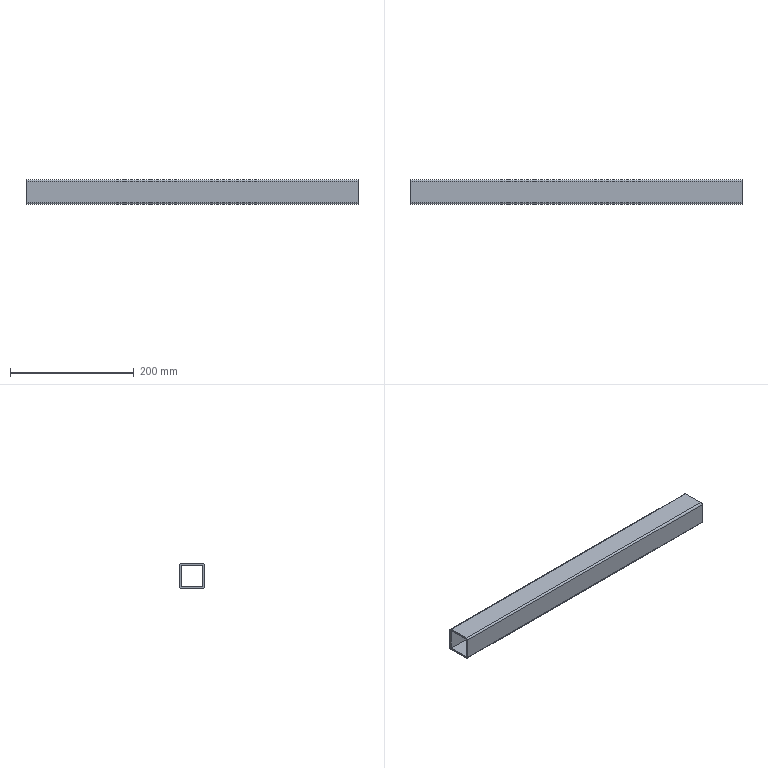Part | NX | features solid 2 | 1 solid | 28 faces | box 536 x 40 x 40 mm | volume 219712 mm3 | plane 24 | cylinder 4 | commonest cylinder face diameters 5.6 x4
STEP:
#1=CARTESIAN_POINT('',(-268.,-42.2,-355.7));
#2=VERTEX_POINT('',#1);
#3=CARTESIAN_POINT('',(-268.,-7.8,-355.7));
#4=VERTEX_POINT('',#3);
#5=CARTESIAN_POINT('',(-268.,-42.2,-355.7));
#6=DIRECTION('',(0.,1.,0.));
#7=VECTOR('',#6,1000.);
#8=LINE('',#5,#7);
#9=EDGE_CURVE('',#2,#4,#8,.T.);
#10=ORIENTED_EDGE('',*,*,#9,.T.);
#11=CARTESIAN_POINT('',(268.,-7.8,-355.7));
#12=VERTEX_POINT('',#11);
#13=CARTESIAN_POINT('',(-268.,-7.8,-355.7));
#14=DIRECTION('',(1.,0.,0.));
#15=VECTOR('',#14,1000.);
#16=LINE('',#13,#15);
#17=EDGE_CURVE('',#4,#12,#16,.T.);
#18=ORIENTED_EDGE('',*,*,#17,.T.);
#19=CARTESIAN_POINT('',(268.,-42.2,-355.7));
#20=VERTEX_POINT('',#19);
#21=CARTESIAN_POINT('',(268.,-42.2,-355.7));
#22=DIRECTION('',(0.,1.,0.));
#23=VECTOR('',#22,1000.);
#24=LINE('',#21,#23);
#25=EDGE_CURVE('',#20,#12,#24,.T.);
#26=ORIENTED_EDGE('',*,*,#25,.F.);
#27=CARTESIAN_POINT('',(268.,-42.2,-355.7));
#28=DIRECTION('',(-1.,0.,0.));
#29=VECTOR('',#28,1000.);
#30=LINE('',#27,#29);
#31=EDGE_CURVE('',#20,#2,#30,.T.);
#32=ORIENTED_EDGE('',*,*,#31,.T.);
#33=EDGE_LOOP('',(#10,#18,#26,#32));
#34=FACE_BOUND('',#33,.T.);
#35=CARTESIAN_POINT('',(-268.,-45.,-355.7));
#36=DIRECTION('',(0.,0.,-1.));
#37=DIRECTION('',(0.,-1.,0.));
#38=AXIS2_PLACEMENT_3D('',#35,#36,#37);
#39=PLANE('',#38);
#40=ADVANCED_FACE('',(#34),#39,.T.);
#41=CARTESIAN_POINT('',(-268.,-45.,-352.9));
#42=VERTEX_POINT('',#41);
#43=CARTESIAN_POINT('',(-268.,-42.2,-352.9));
#44=DIRECTION('',(1.,0.,0.));
#45=DIRECTION('',(0.,-1.,0.));
#46=AXIS2_PLACEMENT_3D('',#43,#44,#45);
#47=CIRCLE('',#46,2.8);
#48=EDGE_CURVE('',#42,#2,#47,.T.);
#49=ORIENTED_EDGE('',*,*,#48,.T.);
#50=ORIENTED_EDGE('',*,*,#31,.F.);
#51=CARTESIAN_POINT('',(268.,-45.,-352.9));
#52=VERTEX_POINT('',#51);
#53=CARTESIAN_POINT('',(268.,-42.2,-352.9));
#54=DIRECTION('',(-1.,0.,0.));
#55=DIRECTION('',(0.,0.,-1.));
#56=AXIS2_PLACEMENT_3D('',#53,#54,#55);
#57=CIRCLE('',#56,2.8);
#58=EDGE_CURVE('',#20,#52,#57,.T.);
#59=ORIENTED_EDGE('',*,*,#58,.T.);
#60=CARTESIAN_POINT('',(-268.,-45.,-352.9));
#61=DIRECTION('',(1.,0.,0.));
#62=VECTOR('',#61,1000.);
#63=LINE('',#60,#62);
#64=EDGE_CURVE('',#42,#52,#63,.T.);
#65=ORIENTED_EDGE('',*,*,#64,.F.);
#66=EDGE_LOOP('',(#49,#50,#59,#65));
#67=FACE_BOUND('',#66,.T.);
#68=CARTESIAN_POINT('',(966.73,-42.2,-352.9));
#69=DIRECTION('',(-1.,0.,0.));
#70=DIRECTION('',(0.,0.,1.));
#71=AXIS2_PLACEMENT_3D('',#68,#69,#70);
#72=CYLINDRICAL_SURFACE('',#71,2.8);
#73=ADVANCED_FACE('',(#67),#72,.T.);
#74=CARTESIAN_POINT('',(268.,-45.,-318.5));
#75=VERTEX_POINT('',#74);
#76=CARTESIAN_POINT('',(268.,-45.,-318.5));
#77=DIRECTION('',(0.,0.,-1.));
#78=VECTOR('',#77,1000.);
#79=LINE('',#76,#78);
#80=EDGE_CURVE('',#75,#52,#79,.T.);
#81=ORIENTED_EDGE('',*,*,#80,.F.);
#82=CARTESIAN_POINT('',(-268.,-45.,-318.5));
#83=VERTEX_POINT('',#82);
#84=CARTESIAN_POINT('',(268.,-45.,-318.5));
#85=DIRECTION('',(-1.,0.,0.));
#86=VECTOR('',#85,1000.);
#87=LINE('',#84,#86);
#88=EDGE_CURVE('',#75,#83,#87,.T.);
#89=ORIENTED_EDGE('',*,*,#88,.T.);
#90=CARTESIAN_POINT('',(-268.,-45.,-318.5));
#91=DIRECTION('',(0.,0.,-1.));
#92=VECTOR('',#91,1000.);
#93=LINE('',#90,#92);
#94=EDGE_CURVE('',#83,#42,#93,.T.);
#95=ORIENTED_EDGE('',*,*,#94,.T.);
#96=ORIENTED_EDGE('',*,*,#64,.T.);
#97=EDGE_LOOP('',(#81,#89,#95,#96));
#98=FACE_BOUND('',#97,.T.);
#99=CARTESIAN_POINT('',(-268.,-45.,-315.7));
#100=DIRECTION('',(0.,-1.,0.));
#101=DIRECTION('',(0.,0.,1.));
#102=AXIS2_PLACEMENT_3D('',#99,#100,#101);
#103=PLANE('',#102);
#104=ADVANCED_FACE('',(#98),#103,.T.);
#105=ORIENTED_EDGE('',*,*,#94,.F.);
#106=CARTESIAN_POINT('',(-268.,-42.2,-318.5));
#107=VERTEX_POINT('',#106);
#108=CARTESIAN_POINT('',(-268.,-45.,-318.5));
#109=DIRECTION('',(0.,1.,0.));
#110=VECTOR('',#109,1000.);
#111=LINE('',#108,#110);
#112=EDGE_CURVE('',#83,#107,#111,.T.);
#113=ORIENTED_EDGE('',*,*,#112,.T.);
#114=CARTESIAN_POINT('',(-268.,-42.2,-352.9));
#115=VERTEX_POINT('',#114);
#116=CARTESIAN_POINT('',(-268.,-42.2,-318.5));
#117=DIRECTION('',(0.,0.,-1.));
#118=VECTOR('',#117,1000.);
#119=LINE('',#116,#118);
#120=EDGE_CURVE('',#107,#115,#119,.T.);
#121=ORIENTED_EDGE('',*,*,#120,.T.);
#122=CARTESIAN_POINT('',(-268.,-45.,-352.9));
#123=DIRECTION('',(0.,1.,0.));
#124=VECTOR('',#123,1000.);
#125=LINE('',#122,#124);
#126=EDGE_CURVE('',#42,#115,#125,.T.);
#127=ORIENTED_EDGE('',*,*,#126,.F.);
#128=EDGE_LOOP('',(#105,#113,#121,#127));
#129=FACE_BOUND('',#128,.T.);
#130=CARTESIAN_POINT('',(-268.,-43.6,-335.7));
#131=DIRECTION('',(-1.,0.,0.));
#132=DIRECTION('',(0.,0.,1.));
#133=AXIS2_PLACEMENT_3D('',#130,#131,#132);
#134=PLANE('',#133);
#135=ADVANCED_FACE('',(#129),#134,.T.);
#136=ORIENTED_EDGE('',*,*,#126,.T.);
#137=CARTESIAN_POINT('',(-268.,-42.2,-355.7));
#138=DIRECTION('',(0.,0.,1.));
#139=VECTOR('',#138,1000.);
#140=LINE('',#137,#139);
#141=EDGE_CURVE('',#2,#115,#140,.T.);
#142=ORIENTED_EDGE('',*,*,#141,.F.);
#143=ORIENTED_EDGE('',*,*,#48,.F.);
#144=EDGE_LOOP('',(#136,#142,#143));
#145=FACE_BOUND('',#144,.T.);
#146=CARTESIAN_POINT('',(-268.,-43.19,-353.89));
#147=DIRECTION('',(1.,0.,0.));
#148=DIRECTION('',(0.,1.,0.));
#149=AXIS2_PLACEMENT_3D('',#146,#147,#148);
#150=PLANE('',#149);
#151=ADVANCED_FACE('',(#145),#150,.F.);
#152=ORIENTED_EDGE('',*,*,#9,.F.);
#153=ORIENTED_EDGE('',*,*,#141,.T.);
#154=CARTESIAN_POINT('',(-268.,-7.8,-352.9));
#155=VERTEX_POINT('',#154);
#156=CARTESIAN_POINT('',(-268.,-42.2,-352.9));
#157=DIRECTION('',(0.,1.,0.));
#158=VECTOR('',#157,1000.);
#159=LINE('',#156,#158);
#160=EDGE_CURVE('',#115,#155,#159,.T.);
#161=ORIENTED_EDGE('',*,*,#160,.T.);
#162=CARTESIAN_POINT('',(-268.,-7.8,-355.7));
#163=DIRECTION('',(0.,0.,1.));
#164=VECTOR('',#163,1000.);
#165=LINE('',#162,#164);
#166=EDGE_CURVE('',#4,#155,#165,.T.);
#167=ORIENTED_EDGE('',*,*,#166,.F.);
#168=EDGE_LOOP('',(#152,#153,#161,#167));
#169=FACE_BOUND('',#168,.T.);
#170=CARTESIAN_POINT('',(-268.,-25.,-354.3));
#171=DIRECTION('',(-1.,0.,0.));
#172=DIRECTION('',(0.,-1.,0.));
#173=AXIS2_PLACEMENT_3D('',#170,#171,#172);
#174=PLANE('',#173);
#175=ADVANCED_FACE('',(#169),#174,.T.);
#176=ORIENTED_EDGE('',*,*,#166,.T.);
#177=CARTESIAN_POINT('',(-268.,-5.,-352.9));
#178=VERTEX_POINT('',#177);
#179=CARTESIAN_POINT('',(-268.,-5.,-352.9));
#180=DIRECTION('',(0.,-1.,0.));
#181=VECTOR('',#180,1000.);
#182=LINE('',#179,#181);
#183=EDGE_CURVE('',#178,#155,#182,.T.);
#184=ORIENTED_EDGE('',*,*,#183,.F.);
#185=CARTESIAN_POINT('',(-268.,-7.8,-352.9));
#186=DIRECTION('',(1.,0.,0.));
#187=DIRECTION('',(0.,0.,-1.));
#188=AXIS2_PLACEMENT_3D('',#185,#186,#187);
#189=CIRCLE('',#188,2.8);
#190=EDGE_CURVE('',#4,#178,#189,.T.);
#191=ORIENTED_EDGE('',*,*,#190,.F.);
#192=EDGE_LOOP('',(#176,#184,#191));
#193=FACE_BOUND('',#192,.T.);
#194=CARTESIAN_POINT('',(-268.,-6.81,-353.89));
#195=DIRECTION('',(1.,0.,0.));
#196=DIRECTION('',(0.,0.,1.));
#197=AXIS2_PLACEMENT_3D('',#194,#195,#196);
#198=PLANE('',#197);
#199=ADVANCED_FACE('',(#193),#198,.F.);
#200=ORIENTED_EDGE('',*,*,#190,.T.);
#201=CARTESIAN_POINT('',(268.,-5.,-352.9));
#202=VERTEX_POINT('',#201);
#203=CARTESIAN_POINT('',(268.,-5.,-352.9));
#204=DIRECTION('',(-1.,0.,0.));
#205=VECTOR('',#204,1000.);
#206=LINE('',#203,#205);
#207=EDGE_CURVE('',#202,#178,#206,.T.);
#208=ORIENTED_EDGE('',*,*,#207,.F.);
#209=CARTESIAN_POINT('',(268.,-7.8,-352.9));
#210=DIRECTION('',(-1.,0.,0.));
#211=DIRECTION('',(0.,1.,0.));
#212=AXIS2_PLACEMENT_3D('',#209,#210,#211);
#213=CIRCLE('',#212,2.8);
#214=EDGE_CURVE('',#202,#12,#213,.T.);
#215=ORIENTED_EDGE('',*,*,#214,.T.);
#216=ORIENTED_EDGE('',*,*,#17,.F.);
#217=EDGE_LOOP('',(#200,#208,#215,#216));
#218=FACE_BOUND('',#217,.T.);
#219=CARTESIAN_POINT('',(966.73,-7.8,-352.9));
#220=DIRECTION('',(-1.,0.,0.));
#221=DIRECTION('',(0.,-1.,0.));
#222=AXIS2_PLACEMENT_3D('',#219,#220,#221);
#223=CYLINDRICAL_SURFACE('',#222,2.8);
#224=ADVANCED_FACE('',(#218),#223,.T.);
#225=CARTESIAN_POINT('',(268.,-7.8,-352.9));
#226=VERTEX_POINT('',#225);
#227=CARTESIAN_POINT('',(268.,-5.,-352.9));
#228=DIRECTION('',(0.,-1.,0.));
#229=VECTOR('',#228,1000.);
#230=LINE('',#227,#229);
#231=EDGE_CURVE('',#202,#226,#230,.T.);
#232=ORIENTED_EDGE('',*,*,#231,.T.);
#233=CARTESIAN_POINT('',(268.,-7.8,-355.7));
#234=DIRECTION('',(0.,0.,1.));
#235=VECTOR('',#234,1000.);
#236=LINE('',#233,#235);
#237=EDGE_CURVE('',#12,#226,#236,.T.);
#238=ORIENTED_EDGE('',*,*,#237,.F.);
#239=ORIENTED_EDGE('',*,*,#214,.F.);
#240=EDGE_LOOP('',(#232,#238,#239));
#241=FACE_BOUND('',#240,.T.);
#242=CARTESIAN_POINT('',(268.,-6.81,-353.89));
#243=DIRECTION('',(-1.,0.,0.));
#244=DIRECTION('',(0.,-1.,0.));
#245=AXIS2_PLACEMENT_3D('',#242,#243,#244);
#246=PLANE('',#245);
#247=ADVANCED_FACE('',(#241),#246,.F.);
#248=ORIENTED_EDGE('',*,*,#25,.T.);
#249=ORIENTED_EDGE('',*,*,#237,.T.);
#250=CARTESIAN_POINT('',(268.,-42.2,-352.9));
#251=VERTEX_POINT('',#250);
#252=CARTESIAN_POINT('',(268.,-42.2,-352.9));
#253=DIRECTION('',(0.,1.,0.));
#254=VECTOR('',#253,1000.);
#255=LINE('',#252,#254);
#256=EDGE_CURVE('',#251,#226,#255,.T.);
#257=ORIENTED_EDGE('',*,*,#256,.F.);
#258=CARTESIAN_POINT('',(268.,-42.2,-355.7));
#259=DIRECTION('',(0.,0.,1.));
#260=VECTOR('',#259,1000.);
#261=LINE('',#258,#260);
#262=EDGE_CURVE('',#20,#251,#261,.T.);
#263=ORIENTED_EDGE('',*,*,#262,.F.);
#264=EDGE_LOOP('',(#248,#249,#257,#263));
#265=FACE_BOUND('',#264,.T.);
#266=CARTESIAN_POINT('',(268.,-25.,-354.3));
#267=DIRECTION('',(-1.,0.,0.));
#268=DIRECTION('',(0.,-1.,0.));
#269=AXIS2_PLACEMENT_3D('',#266,#267,#268);
#270=PLANE('',#269);
#271=ADVANCED_FACE('',(#265),#270,.F.);
#272=ORIENTED_EDGE('',*,*,#262,.T.);
#273=CARTESIAN_POINT('',(268.,-45.,-352.9));
#274=DIRECTION('',(0.,1.,0.));
#275=VECTOR('',#274,1000.);
#276=LINE('',#273,#275);
#277=EDGE_CURVE('',#52,#251,#276,.T.);
#278=ORIENTED_EDGE('',*,*,#277,.F.);
#279=ORIENTED_EDGE('',*,*,#58,.F.);
#280=EDGE_LOOP('',(#272,#278,#279));
#281=FACE_BOUND('',#280,.T.);
#282=CARTESIAN_POINT('',(268.,-43.19,-353.89));
#283=DIRECTION('',(-1.,0.,0.));
#284=DIRECTION('',(0.,0.,1.));
#285=AXIS2_PLACEMENT_3D('',#282,#283,#284);
#286=PLANE('',#285);
#287=ADVANCED_FACE('',(#281),#286,.F.);
#288=ORIENTED_EDGE('',*,*,#80,.T.);
#289=ORIENTED_EDGE('',*,*,#277,.T.);
#290=CARTESIAN_POINT('',(268.,-42.2,-318.5));
#291=VERTEX_POINT('',#290);
#292=CARTESIAN_POINT('',(268.,-42.2,-318.5));
#293=DIRECTION('',(0.,0.,-1.));
#294=VECTOR('',#293,1000.);
#295=LINE('',#292,#294);
#296=EDGE_CURVE('',#291,#251,#295,.T.);
#297=ORIENTED_EDGE('',*,*,#296,.F.);
#298=CARTESIAN_POINT('',(268.,-45.,-318.5));
#299=DIRECTION('',(0.,1.,0.));
#300=VECTOR('',#299,1000.);
#301=LINE('',#298,#300);
#302=EDGE_CURVE('',#75,#291,#301,.T.);
#303=ORIENTED_EDGE('',*,*,#302,.F.);
#304=EDGE_LOOP('',(#288,#289,#297,#303));
#305=FACE_BOUND('',#304,.T.);
#306=CARTESIAN_POINT('',(268.,-43.6,-335.7));
#307=DIRECTION('',(-1.,0.,0.));
#308=DIRECTION('',(0.,0.,1.));
#309=AXIS2_PLACEMENT_3D('',#306,#307,#308);
#310=PLANE('',#309);
#311=ADVANCED_FACE('',(#305),#310,.F.);
#312=ORIENTED_EDGE('',*,*,#302,.T.);
#313=CARTESIAN_POINT('',(268.,-42.2,-315.7));
#314=VERTEX_POINT('',#313);
#315=CARTESIAN_POINT('',(268.,-42.2,-315.7));
#316=DIRECTION('',(0.,0.,-1.));
#317=VECTOR('',#316,1000.);
#318=LINE('',#315,#317);
#319=EDGE_CURVE('',#314,#291,#318,.T.);
#320=ORIENTED_EDGE('',*,*,#319,.F.);
#321=CARTESIAN_POINT('',(268.,-42.2,-318.5));
#322=DIRECTION('',(-1.,0.,0.));
#323=DIRECTION('',(0.,-1.,0.));
#324=AXIS2_PLACEMENT_3D('',#321,#322,#323);
#325=CIRCLE('',#324,2.8);
#326=EDGE_CURVE('',#75,#314,#325,.T.);
#327=ORIENTED_EDGE('',*,*,#326,.F.);
#328=EDGE_LOOP('',(#312,#320,#327));
#329=FACE_BOUND('',#328,.T.);
#330=CARTESIAN_POINT('',(268.,-43.19,-317.51));
#331=DIRECTION('',(-1.,0.,0.));
#332=DIRECTION('',(0.,1.,0.));
#333=AXIS2_PLACEMENT_3D('',#330,#331,#332);
#334=PLANE('',#333);
#335=ADVANCED_FACE('',(#329),#334,.F.);
#336=CARTESIAN_POINT('',(-268.,-42.2,-315.7));
#337=VERTEX_POINT('',#336);
#338=CARTESIAN_POINT('',(-268.,-42.2,-318.5));
#339=DIRECTION('',(1.,0.,0.));
#340=DIRECTION('',(0.,0.,1.));
#341=AXIS2_PLACEMENT_3D('',#338,#339,#340);
#342=CIRCLE('',#341,2.8);
#343=EDGE_CURVE('',#337,#83,#342,.T.);
#344=ORIENTED_EDGE('',*,*,#343,.T.);
#345=ORIENTED_EDGE('',*,*,#88,.F.);
#346=ORIENTED_EDGE('',*,*,#326,.T.);
#347=CARTESIAN_POINT('',(-268.,-42.2,-315.7));
#348=DIRECTION('',(1.,0.,0.));
#349=VECTOR('',#348,1000.);
#350=LINE('',#347,#349);
#351=EDGE_CURVE('',#337,#314,#350,.T.);
#352=ORIENTED_EDGE('',*,*,#351,.F.);
#353=EDGE_LOOP('',(#344,#345,#346,#352));
#354=FACE_BOUND('',#353,.T.);
#355=CARTESIAN_POINT('',(966.73,-42.2,-318.5));
#356=DIRECTION('',(-1.,0.,0.));
#357=DIRECTION('',(0.,1.,0.));
#358=AXIS2_PLACEMENT_3D('',#355,#356,#357);
#359=CYLINDRICAL_SURFACE('',#358,2.8);
#360=ADVANCED_FACE('',(#354),#359,.T.);
#361=CARTESIAN_POINT('',(268.,-7.8,-315.7));
#362=VERTEX_POINT('',#361);
#363=CARTESIAN_POINT('',(268.,-7.8,-315.7));
#364=DIRECTION('',(0.,-1.,0.));
#365=VECTOR('',#364,1000.);
#366=LINE('',#363,#365);
#367=EDGE_CURVE('',#362,#314,#366,.T.);
#368=ORIENTED_EDGE('',*,*,#367,.F.);
#369=CARTESIAN_POINT('',(-268.,-7.8,-315.7));
#370=VERTEX_POINT('',#369);
#371=CARTESIAN_POINT('',(268.,-7.8,-315.7));
#372=DIRECTION('',(-1.,0.,0.));
#373=VECTOR('',#372,1000.);
#374=LINE('',#371,#373);
#375=EDGE_CURVE('',#362,#370,#374,.T.);
#376=ORIENTED_EDGE('',*,*,#375,.T.);
#377=CARTESIAN_POINT('',(-268.,-7.8,-315.7));
#378=DIRECTION('',(0.,-1.,0.));
#379=VECTOR('',#378,1000.);
#380=LINE('',#377,#379);
#381=EDGE_CURVE('',#370,#337,#380,.T.);
#382=ORIENTED_EDGE('',*,*,#381,.T.);
#383=ORIENTED_EDGE('',*,*,#351,.T.);
#384=EDGE_LOOP('',(#368,#376,#382,#383));
#385=FACE_BOUND('',#384,.T.);
#386=CARTESIAN_POINT('',(-268.,-5.,-315.7));
#387=DIRECTION('',(0.,0.,1.));
#388=DIRECTION('',(0.,1.,0.));
#389=AXIS2_PLACEMENT_3D('',#386,#387,#388);
#390=PLANE('',#389);
#391=ADVANCED_FACE('',(#385),#390,.T.);
#392=ORIENTED_EDGE('',*,*,#381,.F.);
#393=CARTESIAN_POINT('',(-268.,-7.8,-318.5));
#394=VERTEX_POINT('',#393);
#395=CARTESIAN_POINT('',(-268.,-7.8,-315.7));
#396=DIRECTION('',(0.,0.,-1.));
#397=VECTOR('',#396,1000.);
#398=LINE('',#395,#397);
#399=EDGE_CURVE('',#370,#394,#398,.T.);
#400=ORIENTED_EDGE('',*,*,#399,.T.);
#401=CARTESIAN_POINT('',(-268.,-7.8,-318.5));
#402=DIRECTION('',(0.,-1.,0.));
#403=VECTOR('',#402,1000.);
#404=LINE('',#401,#403);
#405=EDGE_CURVE('',#394,#107,#404,.T.);
#406=ORIENTED_EDGE('',*,*,#405,.T.);
#407=CARTESIAN_POINT('',(-268.,-42.2,-315.7));
#408=DIRECTION('',(0.,0.,-1.));
#409=VECTOR('',#408,1000.);
#410=LINE('',#407,#409);
#411=EDGE_CURVE('',#337,#107,#410,.T.);
#412=ORIENTED_EDGE('',*,*,#411,.F.);
#413=EDGE_LOOP('',(#392,#400,#406,#412));
#414=FACE_BOUND('',#413,.T.);
#415=CARTESIAN_POINT('',(-268.,-25.,-317.1));
#416=DIRECTION('',(-1.,0.,0.));
#417=DIRECTION('',(0.,1.,0.));
#418=AXIS2_PLACEMENT_3D('',#415,#416,#417);
#419=PLANE('',#418);
#420=ADVANCED_FACE('',(#414),#419,.T.);
#421=ORIENTED_EDGE('',*,*,#411,.T.);
#422=ORIENTED_EDGE('',*,*,#112,.F.);
#423=ORIENTED_EDGE('',*,*,#343,.F.);
#424=EDGE_LOOP('',(#421,#422,#423));
#425=FACE_BOUND('',#424,.T.);
#426=CARTESIAN_POINT('',(-268.,-43.19,-317.51));
#427=DIRECTION('',(1.,0.,0.));
#428=DIRECTION('',(0.,0.,-1.));
#429=AXIS2_PLACEMENT_3D('',#426,#427,#428);
#430=PLANE('',#429);
#431=ADVANCED_FACE('',(#425),#430,.F.);
#432=ORIENTED_EDGE('',*,*,#405,.F.);
#433=CARTESIAN_POINT('',(268.,-7.8,-318.5));
#434=VERTEX_POINT('',#433);
#435=CARTESIAN_POINT('',(268.,-7.8,-318.5));
#436=DIRECTION('',(-1.,0.,0.));
#437=VECTOR('',#436,1000.);
#438=LINE('',#435,#437);
#439=EDGE_CURVE('',#434,#394,#438,.T.);
#440=ORIENTED_EDGE('',*,*,#439,.F.);
#441=CARTESIAN_POINT('',(268.,-7.8,-318.5));
#442=DIRECTION('',(0.,-1.,0.));
#443=VECTOR('',#442,1000.);
#444=LINE('',#441,#443);
#445=EDGE_CURVE('',#434,#291,#444,.T.);
#446=ORIENTED_EDGE('',*,*,#445,.T.);
#447=CARTESIAN_POINT('',(268.,-42.2,-318.5));
#448=DIRECTION('',(-1.,0.,0.));
#449=VECTOR('',#448,1000.);
#450=LINE('',#447,#449);
#451=EDGE_CURVE('',#291,#107,#450,.T.);
#452=ORIENTED_EDGE('',*,*,#451,.T.);
#453=EDGE_LOOP('',(#432,#440,#446,#452));
#454=FACE_BOUND('',#453,.T.);
#455=CARTESIAN_POINT('',(-268.,-5.,-318.5));
#456=DIRECTION('',(0.,0.,1.));
#457=DIRECTION('',(0.,1.,0.));
#458=AXIS2_PLACEMENT_3D('',#455,#456,#457);
#459=PLANE('',#458);
#460=ADVANCED_FACE('',(#454),#459,.F.);
#461=ORIENTED_EDGE('',*,*,#120,.F.);
#462=ORIENTED_EDGE('',*,*,#451,.F.);
#463=ORIENTED_EDGE('',*,*,#296,.T.);
#464=CARTESIAN_POINT('',(268.,-42.2,-352.9));
#465=DIRECTION('',(-1.,0.,0.));
#466=VECTOR('',#465,1000.);
#467=LINE('',#464,#466);
#468=EDGE_CURVE('',#251,#115,#467,.T.);
#469=ORIENTED_EDGE('',*,*,#468,.T.);
#470=EDGE_LOOP('',(#461,#462,#463,#469));
#471=FACE_BOUND('',#470,.T.);
#472=CARTESIAN_POINT('',(-268.,-42.2,-315.7));
#473=DIRECTION('',(0.,-1.,0.));
#474=DIRECTION('',(0.,0.,1.));
#475=AXIS2_PLACEMENT_3D('',#472,#473,#474);
#476=PLANE('',#475);
#477=ADVANCED_FACE('',(#471),#476,.F.);
#478=ORIENTED_EDGE('',*,*,#256,.T.);
#479=CARTESIAN_POINT('',(268.,-7.8,-352.9));
#480=DIRECTION('',(-1.,0.,0.));
#481=VECTOR('',#480,1000.);
#482=LINE('',#479,#481);
#483=EDGE_CURVE('',#226,#155,#482,.T.);
#484=ORIENTED_EDGE('',*,*,#483,.T.);
#485=ORIENTED_EDGE('',*,*,#160,.F.);
#486=ORIENTED_EDGE('',*,*,#468,.F.);
#487=EDGE_LOOP('',(#478,#484,#485,#486));
#488=FACE_BOUND('',#487,.T.);
#489=CARTESIAN_POINT('',(-268.,-45.,-352.9));
#490=DIRECTION('',(0.,0.,-1.));
#491=DIRECTION('',(0.,-1.,0.));
#492=AXIS2_PLACEMENT_3D('',#489,#490,#491);
#493=PLANE('',#492);
#494=ADVANCED_FACE('',(#488),#493,.F.);
#495=CARTESIAN_POINT('',(268.,-7.8,-352.9));
#496=DIRECTION('',(0.,0.,1.));
#497=VECTOR('',#496,1000.);
#498=LINE('',#495,#497);
#499=EDGE_CURVE('',#226,#434,#498,.T.);
#500=ORIENTED_EDGE('',*,*,#499,.T.);
#501=ORIENTED_EDGE('',*,*,#439,.T.);
#502=CARTESIAN_POINT('',(-268.,-7.8,-352.9));
#503=DIRECTION('',(0.,0.,1.));
#504=VECTOR('',#503,1000.);
#505=LINE('',#502,#504);
#506=EDGE_CURVE('',#155,#394,#505,.T.);
#507=ORIENTED_EDGE('',*,*,#506,.F.);
#508=ORIENTED_EDGE('',*,*,#483,.F.);
#509=EDGE_LOOP('',(#500,#501,#507,#508));
#510=FACE_BOUND('',#509,.T.);
#511=CARTESIAN_POINT('',(-268.,-7.8,-355.7));
#512=DIRECTION('',(0.,1.,0.));
#513=DIRECTION('',(0.,0.,-1.));
#514=AXIS2_PLACEMENT_3D('',#511,#512,#513);
#515=PLANE('',#514);
#516=ADVANCED_FACE('',(#510),#515,.F.);
#517=CARTESIAN_POINT('',(-268.,-5.,-318.5));
#518=VERTEX_POINT('',#517);
#519=CARTESIAN_POINT('',(-268.,-5.,-352.9));
#520=DIRECTION('',(0.,0.,1.));
#521=VECTOR('',#520,1000.);
#522=LINE('',#519,#521);
#523=EDGE_CURVE('',#178,#518,#522,.T.);
#524=ORIENTED_EDGE('',*,*,#523,.F.);
#525=ORIENTED_EDGE('',*,*,#183,.T.);
#526=ORIENTED_EDGE('',*,*,#506,.T.);
#527=CARTESIAN_POINT('',(-268.,-5.,-318.5));
#528=DIRECTION('',(0.,-1.,0.));
#529=VECTOR('',#528,1000.);
#530=LINE('',#527,#529);
#531=EDGE_CURVE('',#518,#394,#530,.T.);
#532=ORIENTED_EDGE('',*,*,#531,.F.);
#533=EDGE_LOOP('',(#524,#525,#526,#532));
#534=FACE_BOUND('',#533,.T.);
#535=CARTESIAN_POINT('',(-268.,-6.4,-335.7));
#536=DIRECTION('',(-1.,0.,0.));
#537=DIRECTION('',(0.,0.,-1.));
#538=AXIS2_PLACEMENT_3D('',#535,#536,#537);
#539=PLANE('',#538);
#540=ADVANCED_FACE('',(#534),#539,.T.);
#541=ORIENTED_EDGE('',*,*,#531,.T.);
#542=ORIENTED_EDGE('',*,*,#399,.F.);
#543=CARTESIAN_POINT('',(-268.,-7.8,-318.5));
#544=DIRECTION('',(1.,0.,0.));
#545=DIRECTION('',(0.,1.,0.));
#546=AXIS2_PLACEMENT_3D('',#543,#544,#545);
#547=CIRCLE('',#546,2.8);
#548=EDGE_CURVE('',#518,#370,#547,.T.);
#549=ORIENTED_EDGE('',*,*,#548,.F.);
#550=EDGE_LOOP('',(#541,#542,#549));
#551=FACE_BOUND('',#550,.T.);
#552=CARTESIAN_POINT('',(-268.,-6.81,-317.51));
#553=DIRECTION('',(1.,0.,0.));
#554=DIRECTION('',(0.,-1.,0.));
#555=AXIS2_PLACEMENT_3D('',#552,#553,#554);
#556=PLANE('',#555);
#557=ADVANCED_FACE('',(#551),#556,.F.);
#558=ORIENTED_EDGE('',*,*,#548,.T.);
#559=ORIENTED_EDGE('',*,*,#375,.F.);
#560=CARTESIAN_POINT('',(268.,-5.,-318.5));
#561=VERTEX_POINT('',#560);
#562=CARTESIAN_POINT('',(268.,-7.8,-318.5));
#563=DIRECTION('',(-1.,0.,0.));
#564=DIRECTION('',(0.,0.,1.));
#565=AXIS2_PLACEMENT_3D('',#562,#563,#564);
#566=CIRCLE('',#565,2.8);
#567=EDGE_CURVE('',#362,#561,#566,.T.);
#568=ORIENTED_EDGE('',*,*,#567,.T.);
#569=CARTESIAN_POINT('',(-268.,-5.,-318.5));
#570=DIRECTION('',(1.,0.,0.));
#571=VECTOR('',#570,1000.);
#572=LINE('',#569,#571);
#573=EDGE_CURVE('',#518,#561,#572,.T.);
#574=ORIENTED_EDGE('',*,*,#573,.F.);
#575=EDGE_LOOP('',(#558,#559,#568,#574));
#576=FACE_BOUND('',#575,.T.);
#577=CARTESIAN_POINT('',(966.73,-7.8,-318.5));
#578=DIRECTION('',(-1.,0.,0.));
#579=DIRECTION('',(0.,0.,-1.));
#580=AXIS2_PLACEMENT_3D('',#577,#578,#579);
#581=CYLINDRICAL_SURFACE('',#580,2.8);
#582=ADVANCED_FACE('',(#576),#581,.T.);
#583=ORIENTED_EDGE('',*,*,#523,.T.);
#584=ORIENTED_EDGE('',*,*,#573,.T.);
#585=CARTESIAN_POINT('',(268.,-5.,-352.9));
#586=DIRECTION('',(0.,0.,1.));
#587=VECTOR('',#586,1000.);
#588=LINE('',#585,#587);
#589=EDGE_CURVE('',#202,#561,#588,.T.);
#590=ORIENTED_EDGE('',*,*,#589,.F.);
#591=ORIENTED_EDGE('',*,*,#207,.T.);
#592=EDGE_LOOP('',(#583,#584,#590,#591));
#593=FACE_BOUND('',#592,.T.);
#594=CARTESIAN_POINT('',(-268.,-5.,-355.7));
#595=DIRECTION('',(0.,1.,0.));
#596=DIRECTION('',(0.,0.,-1.));
#597=AXIS2_PLACEMENT_3D('',#594,#595,#596);
#598=PLANE('',#597);
#599=ADVANCED_FACE('',(#593),#598,.T.);
#600=ORIENTED_EDGE('',*,*,#589,.T.);
#601=CARTESIAN_POINT('',(268.,-5.,-318.5));
#602=DIRECTION('',(0.,-1.,0.));
#603=VECTOR('',#602,1000.);
#604=LINE('',#601,#603);
#605=EDGE_CURVE('',#561,#434,#604,.T.);
#606=ORIENTED_EDGE('',*,*,#605,.T.);
#607=ORIENTED_EDGE('',*,*,#499,.F.);
#608=ORIENTED_EDGE('',*,*,#231,.F.);
#609=EDGE_LOOP('',(#600,#606,#607,#608));
#610=FACE_BOUND('',#609,.T.);
#611=CARTESIAN_POINT('',(268.,-6.4,-335.7));
#612=DIRECTION('',(-1.,0.,0.));
#613=DIRECTION('',(0.,0.,-1.));
#614=AXIS2_PLACEMENT_3D('',#611,#612,#613);
#615=PLANE('',#614);
#616=ADVANCED_FACE('',(#610),#615,.F.);
#617=CARTESIAN_POINT('',(268.,-7.8,-315.7));
#618=DIRECTION('',(0.,0.,-1.));
#619=VECTOR('',#618,1000.);
#620=LINE('',#617,#619);
#621=EDGE_CURVE('',#362,#434,#620,.T.);
#622=ORIENTED_EDGE('',*,*,#621,.T.);
#623=ORIENTED_EDGE('',*,*,#605,.F.);
#624=ORIENTED_EDGE('',*,*,#567,.F.);
#625=EDGE_LOOP('',(#622,#623,#624));
#626=FACE_BOUND('',#625,.T.);
#627=CARTESIAN_POINT('',(268.,-6.81,-317.51));
#628=DIRECTION('',(-1.,0.,0.));
#629=DIRECTION('',(0.,0.,-1.));
#630=AXIS2_PLACEMENT_3D('',#627,#628,#629);
#631=PLANE('',#630);
#632=ADVANCED_FACE('',(#626),#631,.F.);
#633=ORIENTED_EDGE('',*,*,#367,.T.);
#634=ORIENTED_EDGE('',*,*,#319,.T.);
#635=ORIENTED_EDGE('',*,*,#445,.F.);
#636=ORIENTED_EDGE('',*,*,#621,.F.);
#637=EDGE_LOOP('',(#633,#634,#635,#636));
#638=FACE_BOUND('',#637,.T.);
#639=CARTESIAN_POINT('',(268.,-25.,-317.1));
#640=DIRECTION('',(-1.,0.,0.));
#641=DIRECTION('',(0.,1.,0.));
#642=AXIS2_PLACEMENT_3D('',#639,#640,#641);
#643=PLANE('',#642);
#644=ADVANCED_FACE('',(#638),#643,.F.);
#645=CLOSED_SHELL('',(#40,#73,#104,#135,#151,#175,#199,#224,#247,#271,#287,#311,#335,#360,#391,#420,#431,#460,#477,#494,#516,#540,#557,#582,#599,#616,#632,#644));
#646=MANIFOLD_SOLID_BREP('',#645);
#647=(LENGTH_UNIT()NAMED_UNIT(*)SI_UNIT(.MILLI.,.METRE.));
#648=UNCERTAINTY_MEASURE_WITH_UNIT(LENGTH_MEASURE(0.00001),#647,'','');
#649=(NAMED_UNIT(*)PLANE_ANGLE_UNIT()SI_UNIT($,.RADIAN.));
#650=(NAMED_UNIT(*)SI_UNIT($,.STERADIAN.)SOLID_ANGLE_UNIT());
#651=(GEOMETRIC_REPRESENTATION_CONTEXT(3)GLOBAL_UNCERTAINTY_ASSIGNED_CONTEXT((#648))GLOBAL_UNIT_ASSIGNED_CONTEXT((#647,#649,#650))REPRESENTATION_CONTEXT('',''));
#652=ADVANCED_BREP_SHAPE_REPRESENTATION('',(#646),#651);